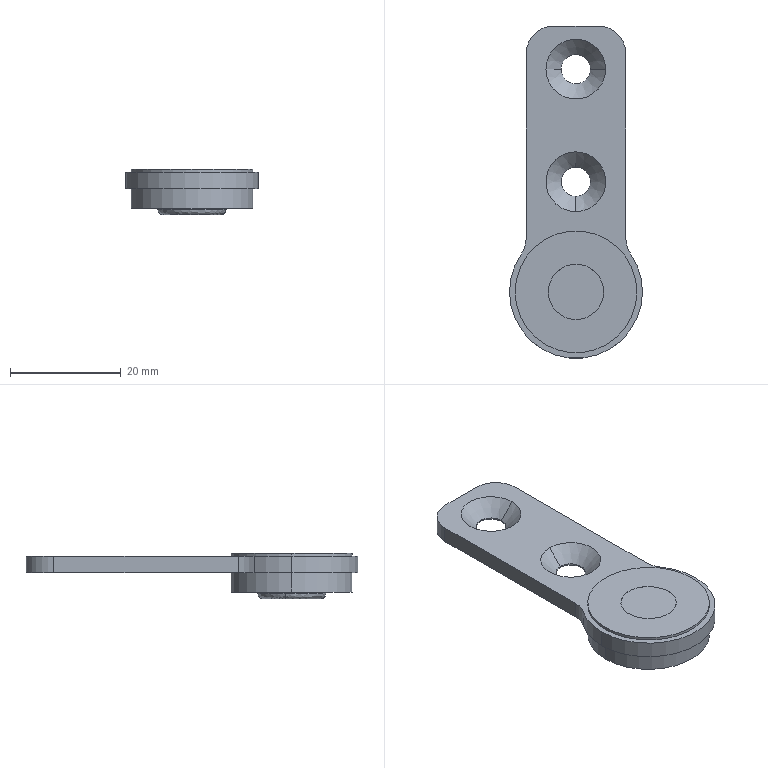Part | SolidWorks | features BaseBody 1 | 1 solid | 43 faces | box 24 x 60 x 8.2 mm | volume 4435 mm3 | cylinder 23 | plane 10 | cone 6 | spline 4 | commonest cylinder face diameters 10 x6 5.3 x4 22 x4 24 x3 7.6 x2 10.02 x2
STEP:
#1=CARTESIAN_POINT('',(-6.03,1.21,-3.8));
#2=VERTEX_POINT('',#1);
#3=CARTESIAN_POINT('',(-6.15,0.,-3.8));
#4=VERTEX_POINT('',#3);
#5=CARTESIAN_POINT('',(0.,0.,-3.8));
#6=DIRECTION('',(0.,0.,1.));
#7=DIRECTION('',(1.,0.,0.));
#8=AXIS2_PLACEMENT_3D('',#5,#6,#7);
#9=CIRCLE('',#8,6.15);
#10=EDGE_CURVE('',#2,#4,#9,.T.);
#11=ORIENTED_EDGE('',*,*,#10,.F.);
#12=CARTESIAN_POINT('',(-5.147,1.033,-4.7));
#13=VERTEX_POINT('',#12);
#14=CARTESIAN_POINT('',(-5.147,1.033,-3.8));
#15=DIRECTION('',(-0.1968,-0.9804,0.));
#16=DIRECTION('',(-0.9804,0.1968,0.));
#17=AXIS2_PLACEMENT_3D('',#14,#15,#16);
#18=CIRCLE('',#17,0.9);
#19=EDGE_CURVE('',#2,#13,#18,.T.);
#20=ORIENTED_EDGE('',*,*,#19,.T.);
#21=CARTESIAN_POINT('',(5.147,-1.033,-4.7));
#22=VERTEX_POINT('',#21);
#23=CARTESIAN_POINT('',(-5.147,1.033,-4.7));
#24=CARTESIAN_POINT('',(-7.214,-9.261,-4.7));
#25=CARTESIAN_POINT('',(3.081,-11.328,-4.7));
#26=CARTESIAN_POINT('',(5.147,-1.033,-4.7));
#27=(BOUNDED_CURVE()B_SPLINE_CURVE(3,(#23,#24,#25,#26),.UNSPECIFIED.,.F.,.F.)B_SPLINE_CURVE_WITH_KNOTS((4,4),(0.,1.),.UNSPECIFIED.)CURVE()GEOMETRIC_REPRESENTATION_ITEM()RATIONAL_B_SPLINE_CURVE((1.,0.3333,0.3333,1.))REPRESENTATION_ITEM(''));
#28=EDGE_CURVE('',#13,#22,#27,.T.);
#29=ORIENTED_EDGE('',*,*,#28,.T.);
#30=CARTESIAN_POINT('',(6.03,-1.21,-3.8));
#31=VERTEX_POINT('',#30);
#32=CARTESIAN_POINT('',(5.147,-1.033,-3.8));
#33=DIRECTION('',(0.1968,0.9804,0.));
#34=DIRECTION('',(0.9804,-0.1968,0.));
#35=AXIS2_PLACEMENT_3D('',#32,#33,#34);
#36=CIRCLE('',#35,0.9);
#37=EDGE_CURVE('',#31,#22,#36,.T.);
#38=ORIENTED_EDGE('',*,*,#37,.F.);
#39=CARTESIAN_POINT('',(0.,0.,-3.8));
#40=DIRECTION('',(0.,0.,1.));
#41=DIRECTION('',(1.,0.,0.));
#42=AXIS2_PLACEMENT_3D('',#39,#40,#41);
#43=CIRCLE('',#42,6.15);
#44=EDGE_CURVE('',#4,#31,#43,.T.);
#45=ORIENTED_EDGE('',*,*,#44,.F.);
#46=EDGE_LOOP('',(#11,#20,#29,#38,#45));
#47=FACE_OUTER_BOUND('',#46,.T.);
#48=CARTESIAN_POINT('',(-6.03,1.21,-3.8));
#49=CARTESIAN_POINT('',(-8.451,-10.849,-3.8));
#50=CARTESIAN_POINT('',(3.609,-13.27,-3.8));
#51=CARTESIAN_POINT('',(6.03,-1.21,-3.8));
#52=CARTESIAN_POINT('',(-6.03,1.21,-4.327));
#53=CARTESIAN_POINT('',(-8.451,-10.849,-4.327));
#54=CARTESIAN_POINT('',(3.609,-13.27,-4.327));
#55=CARTESIAN_POINT('',(6.03,-1.21,-4.327));
#56=CARTESIAN_POINT('',(-5.664,1.137,-4.7));
#57=CARTESIAN_POINT('',(-7.938,-10.191,-4.7));
#58=CARTESIAN_POINT('',(3.39,-12.465,-4.7));
#59=CARTESIAN_POINT('',(5.664,-1.137,-4.7));
#60=CARTESIAN_POINT('',(-5.147,1.033,-4.7));
#61=CARTESIAN_POINT('',(-7.214,-9.261,-4.7));
#62=CARTESIAN_POINT('',(3.081,-11.328,-4.7));
#63=CARTESIAN_POINT('',(5.147,-1.033,-4.7));
#64=(BOUNDED_SURFACE()B_SPLINE_SURFACE(3,3,((#48,#49,#50,#51),(#52,#53,#54,#55),(#56,#57,#58,#59),(#60,#61,#62,#63)),.UNSPECIFIED.,.F.,.F.,.F.)B_SPLINE_SURFACE_WITH_KNOTS((4,4),(4,4),(0.,1.),(0.,1.),.UNSPECIFIED.)GEOMETRIC_REPRESENTATION_ITEM()RATIONAL_B_SPLINE_SURFACE(((1.,0.3333,0.3333,1.),(0.8047,0.2682,0.2682,0.8047),(0.8047,0.2682,0.2682,0.8047),(1.,0.3333,0.3333,1.)))REPRESENTATION_ITEM('')SURFACE());
#65=ADVANCED_FACE('',(#47),#64,.T.);
#66=CARTESIAN_POINT('',(4.608,-0.925,-4.7));
#67=VERTEX_POINT('',#66);
#68=CARTESIAN_POINT('',(-4.608,0.925,-4.7));
#69=VERTEX_POINT('',#68);
#70=CARTESIAN_POINT('',(4.608,-0.925,-4.7));
#71=CARTESIAN_POINT('',(2.758,-10.141,-4.7));
#72=CARTESIAN_POINT('',(-6.458,-8.291,-4.7));
#73=CARTESIAN_POINT('',(-4.608,0.925,-4.7));
#74=(BOUNDED_CURVE()B_SPLINE_CURVE(3,(#70,#71,#72,#73),.UNSPECIFIED.,.F.,.F.)B_SPLINE_CURVE_WITH_KNOTS((4,4),(0.,1.),.UNSPECIFIED.)CURVE()GEOMETRIC_REPRESENTATION_ITEM()RATIONAL_B_SPLINE_CURVE((1.,0.3333,0.3333,1.))REPRESENTATION_ITEM(''));
#75=EDGE_CURVE('',#67,#69,#74,.T.);
#76=ORIENTED_EDGE('',*,*,#75,.T.);
#77=CARTESIAN_POINT('',(-3.726,0.7479,-3.8));
#78=VERTEX_POINT('',#77);
#79=CARTESIAN_POINT('',(-4.608,0.925,-3.8));
#80=DIRECTION('',(-0.1968,-0.9804,0.));
#81=DIRECTION('',(-0.9804,0.1968,0.));
#82=AXIS2_PLACEMENT_3D('',#79,#80,#81);
#83=CIRCLE('',#82,0.9);
#84=EDGE_CURVE('',#69,#78,#83,.T.);
#85=ORIENTED_EDGE('',*,*,#84,.T.);
#86=CARTESIAN_POINT('',(-3.8,0.,-3.8));
#87=VERTEX_POINT('',#86);
#88=CARTESIAN_POINT('',(0.,0.,-3.8));
#89=DIRECTION('',(0.,0.,1.));
#90=DIRECTION('',(0.9804,-0.1968,0.));
#91=AXIS2_PLACEMENT_3D('',#88,#89,#90);
#92=CIRCLE('',#91,3.8);
#93=EDGE_CURVE('',#78,#87,#92,.T.);
#94=ORIENTED_EDGE('',*,*,#93,.T.);
#95=CARTESIAN_POINT('',(3.726,-0.7479,-3.8));
#96=VERTEX_POINT('',#95);
#97=CARTESIAN_POINT('',(0.,0.,-3.8));
#98=DIRECTION('',(0.,0.,1.));
#99=DIRECTION('',(0.9804,-0.1968,0.));
#100=AXIS2_PLACEMENT_3D('',#97,#98,#99);
#101=CIRCLE('',#100,3.8);
#102=EDGE_CURVE('',#87,#96,#101,.T.);
#103=ORIENTED_EDGE('',*,*,#102,.T.);
#104=CARTESIAN_POINT('',(4.608,-0.925,-3.8));
#105=DIRECTION('',(0.1968,0.9804,0.));
#106=DIRECTION('',(0.9804,-0.1968,0.));
#107=AXIS2_PLACEMENT_3D('',#104,#105,#106);
#108=CIRCLE('',#107,0.9);
#109=EDGE_CURVE('',#67,#96,#108,.T.);
#110=ORIENTED_EDGE('',*,*,#109,.F.);
#111=EDGE_LOOP('',(#76,#85,#94,#103,#110));
#112=FACE_OUTER_BOUND('',#111,.T.);
#113=CARTESIAN_POINT('',(-4.608,0.925,-4.7));
#114=CARTESIAN_POINT('',(-6.458,-8.291,-4.7));
#115=CARTESIAN_POINT('',(2.758,-10.141,-4.7));
#116=CARTESIAN_POINT('',(4.608,-0.925,-4.7));
#117=CARTESIAN_POINT('',(-4.091,0.8213,-4.7));
#118=CARTESIAN_POINT('',(-5.734,-7.361,-4.7));
#119=CARTESIAN_POINT('',(2.449,-9.004,-4.7));
#120=CARTESIAN_POINT('',(4.091,-0.8213,-4.7));
#121=CARTESIAN_POINT('',(-3.726,0.7479,-4.327));
#122=CARTESIAN_POINT('',(-5.221,-6.703,-4.327));
#123=CARTESIAN_POINT('',(2.23,-8.199,-4.327));
#124=CARTESIAN_POINT('',(3.726,-0.7479,-4.327));
#125=CARTESIAN_POINT('',(-3.726,0.7479,-3.8));
#126=CARTESIAN_POINT('',(-5.221,-6.703,-3.8));
#127=CARTESIAN_POINT('',(2.23,-8.199,-3.8));
#128=CARTESIAN_POINT('',(3.726,-0.7479,-3.8));
#129=(BOUNDED_SURFACE()B_SPLINE_SURFACE(3,3,((#113,#114,#115,#116),(#117,#118,#119,#120),(#121,#122,#123,#124),(#125,#126,#127,#128)),.UNSPECIFIED.,.F.,.F.,.T.)B_SPLINE_SURFACE_WITH_KNOTS((4,4),(4,4),(0.,1.),(0.,1.),.UNSPECIFIED.)GEOMETRIC_REPRESENTATION_ITEM()RATIONAL_B_SPLINE_SURFACE(((1.,0.3333,0.3333,1.),(0.8047,0.2682,0.2682,0.8047),(0.8047,0.2682,0.2682,0.8047),(1.,0.3333,0.3333,1.)))REPRESENTATION_ITEM('')SURFACE());
#130=ADVANCED_FACE('',(#112),#129,.T.);
#131=CARTESIAN_POINT('',(2.612,40.201,0.));
#132=VERTEX_POINT('',#131);
#133=CARTESIAN_POINT('',(-2.688,40.201,0.));
#134=VERTEX_POINT('',#133);
#135=CARTESIAN_POINT('',(-0.03816,40.201,0.));
#136=DIRECTION('',(0.,0.,-1.));
#137=DIRECTION('',(1.,0.,0.));
#138=AXIS2_PLACEMENT_3D('',#135,#136,#137);
#139=CIRCLE('',#138,2.65);
#140=EDGE_CURVE('',#132,#134,#139,.T.);
#141=ORIENTED_EDGE('',*,*,#140,.T.);
#142=CARTESIAN_POINT('',(-2.688,40.201,0.25));
#143=VERTEX_POINT('',#142);
#144=CARTESIAN_POINT('',(-2.688,40.201,3.));
#145=DIRECTION('',(0.,0.,1.));
#146=VECTOR('',#145,1000.);
#147=LINE('',#144,#146);
#148=EDGE_CURVE('',#134,#143,#147,.T.);
#149=ORIENTED_EDGE('',*,*,#148,.T.);
#150=CARTESIAN_POINT('',(2.612,40.201,0.25));
#151=VERTEX_POINT('',#150);
#152=CARTESIAN_POINT('',(-0.03816,40.201,0.25));
#153=DIRECTION('',(0.,0.,-1.));
#154=DIRECTION('',(1.,0.,0.));
#155=AXIS2_PLACEMENT_3D('',#152,#153,#154);
#156=CIRCLE('',#155,2.65);
#157=EDGE_CURVE('',#151,#143,#156,.T.);
#158=ORIENTED_EDGE('',*,*,#157,.F.);
#159=CARTESIAN_POINT('',(2.612,40.201,3.));
#160=DIRECTION('',(0.,0.,1.));
#161=VECTOR('',#160,1000.);
#162=LINE('',#159,#161);
#163=EDGE_CURVE('',#132,#151,#162,.T.);
#164=ORIENTED_EDGE('',*,*,#163,.F.);
#165=EDGE_LOOP('',(#141,#149,#158,#164));
#166=FACE_OUTER_BOUND('',#165,.T.);
#167=CARTESIAN_POINT('',(-0.03816,40.201,3.));
#168=DIRECTION('',(0.,0.,1.));
#169=DIRECTION('',(1.,0.,0.));
#170=AXIS2_PLACEMENT_3D('',#167,#168,#169);
#171=CYLINDRICAL_SURFACE('',#170,2.65);
#172=ADVANCED_FACE('',(#166),#171,.F.);
#173=CARTESIAN_POINT('',(2.619,19.883,0.));
#174=VERTEX_POINT('',#173);
#175=CARTESIAN_POINT('',(-2.681,19.883,0.));
#176=VERTEX_POINT('',#175);
#177=CARTESIAN_POINT('',(-0.03149,19.883,0.));
#178=DIRECTION('',(0.,0.,-1.));
#179=DIRECTION('',(1.,0.,0.));
#180=AXIS2_PLACEMENT_3D('',#177,#178,#179);
#181=CIRCLE('',#180,2.65);
#182=EDGE_CURVE('',#174,#176,#181,.T.);
#183=ORIENTED_EDGE('',*,*,#182,.T.);
#184=CARTESIAN_POINT('',(-2.681,19.883,0.25));
#185=VERTEX_POINT('',#184);
#186=CARTESIAN_POINT('',(-2.681,19.883,3.));
#187=DIRECTION('',(0.,0.,1.));
#188=VECTOR('',#187,1000.);
#189=LINE('',#186,#188);
#190=EDGE_CURVE('',#176,#185,#189,.T.);
#191=ORIENTED_EDGE('',*,*,#190,.T.);
#192=CARTESIAN_POINT('',(-0.03149,17.233,0.25));
#193=VERTEX_POINT('',#192);
#194=CARTESIAN_POINT('',(-0.03149,19.883,0.25));
#195=DIRECTION('',(0.,0.,-1.));
#196=DIRECTION('',(1.,0.,0.));
#197=AXIS2_PLACEMENT_3D('',#194,#195,#196);
#198=CIRCLE('',#197,2.65);
#199=EDGE_CURVE('',#193,#185,#198,.T.);
#200=ORIENTED_EDGE('',*,*,#199,.F.);
#201=CARTESIAN_POINT('',(2.619,19.883,0.25));
#202=VERTEX_POINT('',#201);
#203=CARTESIAN_POINT('',(-0.03149,19.883,0.25));
#204=DIRECTION('',(0.,0.,-1.));
#205=DIRECTION('',(1.,0.,0.));
#206=AXIS2_PLACEMENT_3D('',#203,#204,#205);
#207=CIRCLE('',#206,2.65);
#208=EDGE_CURVE('',#202,#193,#207,.T.);
#209=ORIENTED_EDGE('',*,*,#208,.F.);
#210=CARTESIAN_POINT('',(2.619,19.883,3.));
#211=DIRECTION('',(0.,0.,1.));
#212=VECTOR('',#211,1000.);
#213=LINE('',#210,#212);
#214=EDGE_CURVE('',#174,#202,#213,.T.);
#215=ORIENTED_EDGE('',*,*,#214,.F.);
#216=EDGE_LOOP('',(#183,#191,#200,#209,#215));
#217=FACE_OUTER_BOUND('',#216,.T.);
#218=CARTESIAN_POINT('',(-0.03149,19.883,3.));
#219=DIRECTION('',(0.,0.,1.));
#220=DIRECTION('',(1.,0.,0.));
#221=AXIS2_PLACEMENT_3D('',#218,#219,#220);
#222=CYLINDRICAL_SURFACE('',#221,2.65);
#223=ADVANCED_FACE('',(#217),#222,.F.);
#224=CARTESIAN_POINT('',(9.882,6.807,3.));
#225=VERTEX_POINT('',#224);
#226=CARTESIAN_POINT('',(12.,0.,3.));
#227=VERTEX_POINT('',#226);
#228=CARTESIAN_POINT('',(0.,0.,3.));
#229=DIRECTION('',(0.,0.,-1.));
#230=DIRECTION('',(-1.,0.,0.));
#231=AXIS2_PLACEMENT_3D('',#228,#229,#230);
#232=CIRCLE('',#231,12.);
#233=EDGE_CURVE('',#225,#227,#232,.T.);
#234=ORIENTED_EDGE('',*,*,#233,.T.);
#235=CARTESIAN_POINT('',(12.,0.,0.));
#236=VERTEX_POINT('',#235);
#237=CARTESIAN_POINT('',(12.,0.,3.));
#238=DIRECTION('',(0.,0.,-1.));
#239=VECTOR('',#238,1000.);
#240=LINE('',#237,#239);
#241=EDGE_CURVE('',#227,#236,#240,.T.);
#242=ORIENTED_EDGE('',*,*,#241,.T.);
#243=CARTESIAN_POINT('',(9.882,6.807,0.));
#244=VERTEX_POINT('',#243);
#245=CARTESIAN_POINT('',(0.,0.,0.));
#246=DIRECTION('',(0.,0.,1.));
#247=DIRECTION('',(-1.,0.,0.));
#248=AXIS2_PLACEMENT_3D('',#245,#246,#247);
#249=CIRCLE('',#248,12.);
#250=EDGE_CURVE('',#236,#244,#249,.T.);
#251=ORIENTED_EDGE('',*,*,#250,.T.);
#252=CARTESIAN_POINT('',(9.882,6.807,3.));
#253=DIRECTION('',(0.,0.,1.));
#254=VECTOR('',#253,1000.);
#255=LINE('',#252,#254);
#256=EDGE_CURVE('',#244,#225,#255,.T.);
#257=ORIENTED_EDGE('',*,*,#256,.T.);
#258=EDGE_LOOP('',(#234,#242,#251,#257));
#259=FACE_OUTER_BOUND('',#258,.T.);
#260=CARTESIAN_POINT('',(0.,0.,3.));
#261=DIRECTION('',(0.,0.,-1.));
#262=DIRECTION('',(-1.,0.,0.));
#263=AXIS2_PLACEMENT_3D('',#260,#261,#262);
#264=CYLINDRICAL_SURFACE('',#263,12.);
#265=ADVANCED_FACE('',(#259),#264,.T.);
#266=ORIENTED_EDGE('',*,*,#241,.F.);
#267=CARTESIAN_POINT('',(-12.,0.,3.));
#268=VERTEX_POINT('',#267);
#269=CARTESIAN_POINT('',(0.,0.,3.));
#270=DIRECTION('',(0.,0.,-1.));
#271=DIRECTION('',(-1.,0.,0.));
#272=AXIS2_PLACEMENT_3D('',#269,#270,#271);
#273=CIRCLE('',#272,12.);
#274=EDGE_CURVE('',#227,#268,#273,.T.);
#275=ORIENTED_EDGE('',*,*,#274,.T.);
#276=CARTESIAN_POINT('',(-12.,0.,0.));
#277=VERTEX_POINT('',#276);
#278=CARTESIAN_POINT('',(-12.,0.,3.));
#279=DIRECTION('',(0.,0.,-1.));
#280=VECTOR('',#279,1000.);
#281=LINE('',#278,#280);
#282=EDGE_CURVE('',#268,#277,#281,.T.);
#283=ORIENTED_EDGE('',*,*,#282,.T.);
#284=CARTESIAN_POINT('',(0.,0.,0.));
#285=DIRECTION('',(0.,0.,1.));
#286=DIRECTION('',(-1.,0.,0.));
#287=AXIS2_PLACEMENT_3D('',#284,#285,#286);
#288=CIRCLE('',#287,12.);
#289=EDGE_CURVE('',#277,#236,#288,.T.);
#290=ORIENTED_EDGE('',*,*,#289,.T.);
#291=EDGE_LOOP('',(#266,#275,#283,#290));
#292=FACE_OUTER_BOUND('',#291,.T.);
#293=CARTESIAN_POINT('',(0.,0.,3.));
#294=DIRECTION('',(0.,0.,-1.));
#295=DIRECTION('',(-1.,0.,0.));
#296=AXIS2_PLACEMENT_3D('',#293,#294,#295);
#297=CYLINDRICAL_SURFACE('',#296,12.);
#298=ADVANCED_FACE('',(#292),#297,.T.);
#299=CARTESIAN_POINT('',(-11.,0.,0.));
#300=VERTEX_POINT('',#299);
#301=CARTESIAN_POINT('',(11.,0.,0.));
#302=VERTEX_POINT('',#301);
#303=CARTESIAN_POINT('',(0.,0.,0.));
#304=DIRECTION('',(0.,0.,-1.));
#305=DIRECTION('',(-1.,0.,0.));
#306=AXIS2_PLACEMENT_3D('',#303,#304,#305);
#307=CIRCLE('',#306,11.);
#308=EDGE_CURVE('',#300,#302,#307,.T.);
#309=ORIENTED_EDGE('',*,*,#308,.T.);
#310=CARTESIAN_POINT('',(11.,0.,-3.5));
#311=VERTEX_POINT('',#310);
#312=CARTESIAN_POINT('',(11.,0.,0.));
#313=DIRECTION('',(0.,0.,-1.));
#314=VECTOR('',#313,1000.);
#315=LINE('',#312,#314);
#316=EDGE_CURVE('',#302,#311,#315,.T.);
#317=ORIENTED_EDGE('',*,*,#316,.T.);
#318=CARTESIAN_POINT('',(-11.,0.,-3.5));
#319=VERTEX_POINT('',#318);
#320=CARTESIAN_POINT('',(0.,0.,-3.5));
#321=DIRECTION('',(0.,0.,1.));
#322=DIRECTION('',(-1.,0.,0.));
#323=AXIS2_PLACEMENT_3D('',#320,#321,#322);
#324=CIRCLE('',#323,11.);
#325=EDGE_CURVE('',#311,#319,#324,.T.);
#326=ORIENTED_EDGE('',*,*,#325,.T.);
#327=CARTESIAN_POINT('',(-11.,0.,0.));
#328=DIRECTION('',(0.,0.,-1.));
#329=VECTOR('',#328,1000.);
#330=LINE('',#327,#329);
#331=EDGE_CURVE('',#300,#319,#330,.T.);
#332=ORIENTED_EDGE('',*,*,#331,.F.);
#333=EDGE_LOOP('',(#309,#317,#326,#332));
#334=FACE_OUTER_BOUND('',#333,.T.);
#335=CARTESIAN_POINT('',(0.,0.,0.));
#336=DIRECTION('',(0.,0.,-1.));
#337=DIRECTION('',(-1.,0.,0.));
#338=AXIS2_PLACEMENT_3D('',#335,#336,#337);
#339=CYLINDRICAL_SURFACE('',#338,11.);
#340=ADVANCED_FACE('',(#334),#339,.T.);
#341=ORIENTED_EDGE('',*,*,#157,.T.);
#342=CARTESIAN_POINT('',(-5.438,40.201,3.));
#343=VERTEX_POINT('',#342);
#344=CARTESIAN_POINT('',(-5.438,40.201,3.));
#345=DIRECTION('',(-0.7071,0.,0.7071));
#346=VECTOR('',#345,1000.);
#347=LINE('',#344,#346);
#348=EDGE_CURVE('',#143,#343,#347,.T.);
#349=ORIENTED_EDGE('',*,*,#348,.T.);
#350=CARTESIAN_POINT('',(5.362,40.201,3.));
#351=VERTEX_POINT('',#350);
#352=CARTESIAN_POINT('',(-0.03816,40.201,3.));
#353=DIRECTION('',(0.,0.,-1.));
#354=DIRECTION('',(1.,0.,0.));
#355=AXIS2_PLACEMENT_3D('',#352,#353,#354);
#356=CIRCLE('',#355,5.4);
#357=EDGE_CURVE('',#351,#343,#356,.T.);
#358=ORIENTED_EDGE('',*,*,#357,.F.);
#359=CARTESIAN_POINT('',(5.362,40.201,3.));
#360=DIRECTION('',(0.7071,0.,0.7071));
#361=VECTOR('',#360,1000.);
#362=LINE('',#359,#361);
#363=EDGE_CURVE('',#151,#351,#362,.T.);
#364=ORIENTED_EDGE('',*,*,#363,.F.);
#365=EDGE_LOOP('',(#341,#349,#358,#364));
#366=FACE_OUTER_BOUND('',#365,.T.);
#367=CARTESIAN_POINT('',(-0.03816,40.201,3.));
#368=DIRECTION('',(0.,0.,1.));
#369=DIRECTION('',(1.,0.,0.));
#370=AXIS2_PLACEMENT_3D('',#367,#368,#369);
#371=CONICAL_SURFACE('',#370,5.4,0.7854);
#372=ADVANCED_FACE('',(#366),#371,.F.);
#373=ORIENTED_EDGE('',*,*,#199,.T.);
#374=CARTESIAN_POINT('',(-0.03149,22.533,0.25));
#375=VERTEX_POINT('',#374);
#376=CARTESIAN_POINT('',(-0.03149,19.883,0.25));
#377=DIRECTION('',(0.,0.,-1.));
#378=DIRECTION('',(1.,0.,0.));
#379=AXIS2_PLACEMENT_3D('',#376,#377,#378);
#380=CIRCLE('',#379,2.65);
#381=EDGE_CURVE('',#185,#375,#380,.T.);
#382=ORIENTED_EDGE('',*,*,#381,.T.);
#383=CARTESIAN_POINT('',(-0.03149,25.283,3.));
#384=VERTEX_POINT('',#383);
#385=CARTESIAN_POINT('',(-0.03149,25.283,3.));
#386=DIRECTION('',(0.,0.7071,0.7071));
#387=VECTOR('',#386,1000.);
#388=LINE('',#385,#387);
#389=EDGE_CURVE('',#375,#384,#388,.T.);
#390=ORIENTED_EDGE('',*,*,#389,.T.);
#391=CARTESIAN_POINT('',(-0.03149,14.483,3.));
#392=VERTEX_POINT('',#391);
#393=CARTESIAN_POINT('',(-0.03149,19.883,3.));
#394=DIRECTION('',(0.,0.,-1.));
#395=DIRECTION('',(0.,-1.,0.));
#396=AXIS2_PLACEMENT_3D('',#393,#394,#395);
#397=CIRCLE('',#396,5.4);
#398=EDGE_CURVE('',#392,#384,#397,.T.);
#399=ORIENTED_EDGE('',*,*,#398,.F.);
#400=CARTESIAN_POINT('',(-0.03149,14.483,3.));
#401=DIRECTION('',(0.,-0.7071,0.7071));
#402=VECTOR('',#401,1000.);
#403=LINE('',#400,#402);
#404=EDGE_CURVE('',#193,#392,#403,.T.);
#405=ORIENTED_EDGE('',*,*,#404,.F.);
#406=EDGE_LOOP('',(#373,#382,#390,#399,#405));
#407=FACE_OUTER_BOUND('',#406,.T.);
#408=CARTESIAN_POINT('',(-0.03149,19.883,3.));
#409=DIRECTION('',(0.,0.,1.));
#410=DIRECTION('',(0.,-1.,0.));
#411=AXIS2_PLACEMENT_3D('',#408,#409,#410);
#412=CONICAL_SURFACE('',#411,5.4,0.7854);
#413=ADVANCED_FACE('',(#407),#412,.F.);
#414=CARTESIAN_POINT('',(-11.,0.,3.5));
#415=VERTEX_POINT('',#414);
#416=CARTESIAN_POINT('',(11.,0.,3.5));
#417=VERTEX_POINT('',#416);
#418=CARTESIAN_POINT('',(0.,0.,3.5));
#419=DIRECTION('',(0.,0.,-1.));
#420=DIRECTION('',(-1.,0.,0.));
#421=AXIS2_PLACEMENT_3D('',#418,#419,#420);
#422=CIRCLE('',#421,11.);
#423=EDGE_CURVE('',#415,#417,#422,.T.);
#424=ORIENTED_EDGE('',*,*,#423,.T.);
#425=CARTESIAN_POINT('',(11.,0.,3.));
#426=VERTEX_POINT('',#425);
#427=CARTESIAN_POINT('',(11.,0.,3.5));
#428=DIRECTION('',(0.,0.,-1.));
#429=VECTOR('',#428,1000.);
#430=LINE('',#427,#429);
#431=EDGE_CURVE('',#417,#426,#430,.T.);
#432=ORIENTED_EDGE('',*,*,#431,.T.);
#433=CARTESIAN_POINT('',(-11.,0.,3.));
#434=VERTEX_POINT('',#433);
#435=CARTESIAN_POINT('',(0.,0.,3.));
#436=DIRECTION('',(0.,0.,-1.));
#437=DIRECTION('',(-1.,0.,0.));
#438=AXIS2_PLACEMENT_3D('',#435,#436,#437);
#439=CIRCLE('',#438,11.);
#440=EDGE_CURVE('',#434,#426,#439,.T.);
#441=ORIENTED_EDGE('',*,*,#440,.F.);
#442=CARTESIAN_POINT('',(-11.,0.,3.5));
#443=DIRECTION('',(0.,0.,-1.));
#444=VECTOR('',#443,1000.);
#445=LINE('',#442,#444);
#446=EDGE_CURVE('',#415,#434,#445,.T.);
#447=ORIENTED_EDGE('',*,*,#446,.F.);
#448=EDGE_LOOP('',(#424,#432,#441,#447));
#449=FACE_OUTER_BOUND('',#448,.T.);
#450=CARTESIAN_POINT('',(0.,0.,3.5));
#451=DIRECTION('',(0.,0.,-1.));
#452=DIRECTION('',(-1.,0.,0.));
#453=AXIS2_PLACEMENT_3D('',#450,#451,#452);
#454=CYLINDRICAL_SURFACE('',#453,11.);
#455=ADVANCED_FACE('',(#449),#454,.T.);
#456=CARTESIAN_POINT('',(6.15,0.,-3.8));
#457=VERTEX_POINT('',#456);
#458=CARTESIAN_POINT('',(0.,0.,-3.8));
#459=DIRECTION('',(0.,0.,1.));
#460=DIRECTION('',(1.,0.,0.));
#461=AXIS2_PLACEMENT_3D('',#458,#459,#460);
#462=CIRCLE('',#461,6.15);
#463=EDGE_CURVE('',#457,#2,#462,.T.);
#464=ORIENTED_EDGE('',*,*,#463,.T.);
#465=ORIENTED_EDGE('',*,*,#10,.T.);
#466=CARTESIAN_POINT('',(-6.15,0.,-3.5));
#467=VERTEX_POINT('',#466);
#468=CARTESIAN_POINT('',(-6.15,0.,60.062));
#469=DIRECTION('',(0.,0.,1.));
#470=VECTOR('',#469,1000.);
#471=LINE('',#468,#470);
#472=EDGE_CURVE('',#4,#467,#471,.T.);
#473=ORIENTED_EDGE('',*,*,#472,.T.);
#474=CARTESIAN_POINT('',(6.15,0.,-3.5));
#475=VERTEX_POINT('',#474);
#476=CARTESIAN_POINT('',(0.,0.,-3.5));
#477=DIRECTION('',(0.,0.,-1.));
#478=DIRECTION('',(1.,0.,0.));
#479=AXIS2_PLACEMENT_3D('',#476,#477,#478);
#480=CIRCLE('',#479,6.15);
#481=EDGE_CURVE('',#467,#475,#480,.T.);
#482=ORIENTED_EDGE('',*,*,#481,.T.);
#483=CARTESIAN_POINT('',(6.15,0.,60.062));
#484=DIRECTION('',(0.,0.,1.));
#485=VECTOR('',#484,1000.);
#486=LINE('',#483,#485);
#487=EDGE_CURVE('',#457,#475,#486,.T.);
#488=ORIENTED_EDGE('',*,*,#487,.F.);
#489=EDGE_LOOP('',(#464,#465,#473,#482,#488));
#490=FACE_OUTER_BOUND('',#489,.T.);
#491=CARTESIAN_POINT('',(0.,0.,60.062));
#492=DIRECTION('',(0.,0.,1.));
#493=DIRECTION('',(1.,0.,0.));
#494=AXIS2_PLACEMENT_3D('',#491,#492,#493);
#495=CYLINDRICAL_SURFACE('',#494,6.15);
#496=ADVANCED_FACE('',(#490),#495,.T.);
#497=CARTESIAN_POINT('',(-5.01,0.,-3.5));
#498=VERTEX_POINT('',#497);
#499=CARTESIAN_POINT('',(5.01,0.,-3.5));
#500=VERTEX_POINT('',#499);
#501=CARTESIAN_POINT('',(0.,0.,-3.5));
#502=DIRECTION('',(0.,0.,1.));
#503=DIRECTION('',(1.,0.,0.));
#504=AXIS2_PLACEMENT_3D('',#501,#502,#503);
#505=CIRCLE('',#504,5.01);
#506=EDGE_CURVE('',#498,#500,#505,.T.);
#507=ORIENTED_EDGE('',*,*,#506,.F.);
#508=CARTESIAN_POINT('',(-5.01,0.,3.5));
#509=VERTEX_POINT('',#508);
#510=CARTESIAN_POINT('',(-5.01,0.,3.));
#511=DIRECTION('',(0.,0.,1.));
#512=VECTOR('',#511,1000.);
#513=LINE('',#510,#512);
#514=EDGE_CURVE('',#498,#509,#513,.T.);
#515=ORIENTED_EDGE('',*,*,#514,.T.);
#516=CARTESIAN_POINT('',(5.01,0.,3.5));
#517=VERTEX_POINT('',#516);
#518=CARTESIAN_POINT('',(0.,0.,3.5));
#519=DIRECTION('',(0.,0.,-1.));
#520=DIRECTION('',(1.,0.,0.));
#521=AXIS2_PLACEMENT_3D('',#518,#519,#520);
#522=CIRCLE('',#521,5.01);
#523=EDGE_CURVE('',#517,#509,#522,.T.);
#524=ORIENTED_EDGE('',*,*,#523,.F.);
#525=CARTESIAN_POINT('',(5.01,0.,3.));
#526=DIRECTION('',(0.,0.,1.));
#527=VECTOR('',#526,1000.);
#528=LINE('',#525,#527);
#529=EDGE_CURVE('',#500,#517,#528,.T.);
#530=ORIENTED_EDGE('',*,*,#529,.F.);
#531=EDGE_LOOP('',(#507,#515,#524,#530));
#532=FACE_OUTER_BOUND('',#531,.T.);
#533=CARTESIAN_POINT('',(0.,0.,3.));
#534=DIRECTION('',(0.,0.,1.));
#535=DIRECTION('',(1.,0.,0.));
#536=AXIS2_PLACEMENT_3D('',#533,#534,#535);
#537=CYLINDRICAL_SURFACE('',#536,5.01);
#538=ADVANCED_FACE('',(#532),#537,.F.);
#539=CARTESIAN_POINT('',(5.,0.,-3.5));
#540=VERTEX_POINT('',#539);
#541=CARTESIAN_POINT('',(-5.,0.,-3.5));
#542=VERTEX_POINT('',#541);
#543=CARTESIAN_POINT('',(0.,0.,-3.5));
#544=DIRECTION('',(0.,0.,1.));
#545=DIRECTION('',(1.,0.,0.));
#546=AXIS2_PLACEMENT_3D('',#543,#544,#545);
#547=CIRCLE('',#546,5.);
#548=EDGE_CURVE('',#540,#542,#547,.T.);
#549=ORIENTED_EDGE('',*,*,#548,.T.);
#550=CARTESIAN_POINT('',(-5.,0.,3.5));
#551=VERTEX_POINT('',#550);
#552=CARTESIAN_POINT('',(-5.,0.,60.062));
#553=DIRECTION('',(0.,0.,1.));
#554=VECTOR('',#553,1000.);
#555=LINE('',#552,#554);
#556=EDGE_CURVE('',#542,#551,#555,.T.);
#557=ORIENTED_EDGE('',*,*,#556,.T.);
#558=CARTESIAN_POINT('',(5.,0.,3.5));
#559=VERTEX_POINT('',#558);
#560=CARTESIAN_POINT('',(0.,0.,3.5));
#561=DIRECTION('',(0.,0.,-1.));
#562=DIRECTION('',(1.,0.,0.));
#563=AXIS2_PLACEMENT_3D('',#560,#561,#562);
#564=CIRCLE('',#563,5.);
#565=EDGE_CURVE('',#551,#559,#564,.T.);
#566=ORIENTED_EDGE('',*,*,#565,.T.);
#567=CARTESIAN_POINT('',(5.,0.,60.062));
#568=DIRECTION('',(0.,0.,1.));
#569=VECTOR('',#568,1000.);
#570=LINE('',#567,#569);
#571=EDGE_CURVE('',#540,#559,#570,.T.);
#572=ORIENTED_EDGE('',*,*,#571,.F.);
#573=EDGE_LOOP('',(#549,#557,#566,#572));
#574=FACE_OUTER_BOUND('',#573,.T.);
#575=CARTESIAN_POINT('',(0.,0.,60.062));
#576=DIRECTION('',(0.,0.,1.));
#577=DIRECTION('',(1.,0.,0.));
#578=AXIS2_PLACEMENT_3D('',#575,#576,#577);
#579=CYLINDRICAL_SURFACE('',#578,5.);
#580=ADVANCED_FACE('',(#574),#579,.T.);
#581=ORIENTED_EDGE('',*,*,#102,.F.);
#582=CARTESIAN_POINT('',(-3.8,0.,0.1));
#583=VERTEX_POINT('',#582);
#584=CARTESIAN_POINT('',(-3.8,0.,60.062));
#585=DIRECTION('',(0.,0.,1.));
#586=VECTOR('',#585,1000.);
#587=LINE('',#584,#586);
#588=EDGE_CURVE('',#87,#583,#587,.T.);
#589=ORIENTED_EDGE('',*,*,#588,.T.);
#590=CARTESIAN_POINT('',(3.8,0.,0.1));
#591=VERTEX_POINT('',#590);
#592=CARTESIAN_POINT('',(0.,0.,0.1));
#593=DIRECTION('',(0.,0.,-1.));
#594=DIRECTION('',(1.,0.,0.));
#595=AXIS2_PLACEMENT_3D('',#592,#593,#594);
#596=CIRCLE('',#595,3.8);
#597=EDGE_CURVE('',#591,#583,#596,.T.);
#598=ORIENTED_EDGE('',*,*,#597,.F.);
#599=CARTESIAN_POINT('',(3.8,0.,-3.8));
#600=VERTEX_POINT('',#599);
#601=CARTESIAN_POINT('',(3.8,0.,60.062));
#602=DIRECTION('',(0.,0.,1.));
#603=VECTOR('',#602,1000.);
#604=LINE('',#601,#603);
#605=EDGE_CURVE('',#600,#591,#604,.T.);
#606=ORIENTED_EDGE('',*,*,#605,.F.);
#607=CARTESIAN_POINT('',(0.,0.,-3.8));
#608=DIRECTION('',(0.,0.,1.));
#609=DIRECTION('',(0.9804,-0.1968,0.));
#610=AXIS2_PLACEMENT_3D('',#607,#608,#609);
#611=CIRCLE('',#610,3.8);
#612=EDGE_CURVE('',#96,#600,#611,.T.);
#613=ORIENTED_EDGE('',*,*,#612,.F.);
#614=EDGE_LOOP('',(#581,#589,#598,#606,#613));
#615=FACE_OUTER_BOUND('',#614,.T.);
#616=CARTESIAN_POINT('',(0.,0.,60.062));
#617=DIRECTION('',(0.,0.,1.));
#618=DIRECTION('',(1.,0.,0.));
#619=AXIS2_PLACEMENT_3D('',#616,#617,#618);
#620=CYLINDRICAL_SURFACE('',#619,3.8);
#621=ADVANCED_FACE('',(#615),#620,.F.);
#622=CARTESIAN_POINT('',(0.,0.,2.294));
#623=VERTEX_POINT('',#622);
#624=CARTESIAN_POINT('',(-3.8,0.,0.1));
#625=DIRECTION('',(-0.866,0.,-0.5));
#626=VECTOR('',#625,1000.);
#627=LINE('',#624,#626);
#628=EDGE_CURVE('',#623,#583,#627,.T.);
#629=ORIENTED_EDGE('',*,*,#628,.F.);
#630=CARTESIAN_POINT('',(3.8,0.,0.1));
#631=DIRECTION('',(0.866,0.,-0.5));
#632=VECTOR('',#631,1000.);
#633=LINE('',#630,#632);
#634=EDGE_CURVE('',#623,#591,#633,.T.);
#635=ORIENTED_EDGE('',*,*,#634,.T.);
#636=ORIENTED_EDGE('',*,*,#597,.T.);
#637=EDGE_LOOP('',(#629,#635,#636));
#638=FACE_OUTER_BOUND('',#637,.T.);
#639=CARTESIAN_POINT('',(0.,0.,0.1));
#640=DIRECTION('',(0.,0.,-1.));
#641=DIRECTION('',(-1.,0.,0.));
#642=AXIS2_PLACEMENT_3D('',#639,#640,#641);
#643=CONICAL_SURFACE('',#642,3.8,1.047);
#644=ADVANCED_FACE('',(#638),#643,.F.);
#645=ORIENTED_EDGE('',*,*,#140,.F.);
#646=CARTESIAN_POINT('',(-0.03816,40.201,0.));
#647=DIRECTION('',(0.,0.,-1.));
#648=DIRECTION('',(1.,0.,0.));
#649=AXIS2_PLACEMENT_3D('',#646,#647,#648);
#650=CIRCLE('',#649,2.65);
#651=EDGE_CURVE('',#134,#132,#650,.T.);
#652=ORIENTED_EDGE('',*,*,#651,.F.);
#653=EDGE_LOOP('',(#645,#652));
#654=FACE_BOUND('',#653,.T.);
#655=ORIENTED_EDGE('',*,*,#182,.F.);
#656=CARTESIAN_POINT('',(-0.03149,19.883,0.));
#657=DIRECTION('',(0.,0.,-1.));
#658=DIRECTION('',(1.,0.,0.));
#659=AXIS2_PLACEMENT_3D('',#656,#657,#658);
#660=CIRCLE('',#659,2.65);
#661=EDGE_CURVE('',#176,#174,#660,.T.);
#662=ORIENTED_EDGE('',*,*,#661,.F.);
#663=EDGE_LOOP('',(#655,#662));
#664=FACE_BOUND('',#663,.T.);
#665=CARTESIAN_POINT('',(-9.,9.644,0.));
#666=VERTEX_POINT('',#665);
#667=CARTESIAN_POINT('',(-9.882,6.807,0.));
#668=VERTEX_POINT('',#667);
#669=CARTESIAN_POINT('',(-14.,9.644,0.));
#670=DIRECTION('',(0.,0.,-1.));
#671=DIRECTION('',(-1.,0.,0.));
#672=AXIS2_PLACEMENT_3D('',#669,#670,#671);
#673=CIRCLE('',#672,5.);
#674=EDGE_CURVE('',#666,#668,#673,.T.);
#675=ORIENTED_EDGE('',*,*,#674,.F.);
#676=CARTESIAN_POINT('',(-9.,43.,0.));
#677=VERTEX_POINT('',#676);
#678=CARTESIAN_POINT('',(-9.,0.,0.));
#679=DIRECTION('',(0.,-1.,0.));
#680=VECTOR('',#679,1000.);
#681=LINE('',#678,#680);
#682=EDGE_CURVE('',#677,#666,#681,.T.);
#683=ORIENTED_EDGE('',*,*,#682,.F.);
#684=CARTESIAN_POINT('',(-4.,48.,0.));
#685=VERTEX_POINT('',#684);
#686=CARTESIAN_POINT('',(-4.,43.,0.));
#687=DIRECTION('',(0.,0.,1.));
#688=DIRECTION('',(-1.,0.,0.));
#689=AXIS2_PLACEMENT_3D('',#686,#687,#688);
#690=CIRCLE('',#689,5.);
#691=EDGE_CURVE('',#685,#677,#690,.T.);
#692=ORIENTED_EDGE('',*,*,#691,.F.);
#693=CARTESIAN_POINT('',(4.,48.,0.));
#694=VERTEX_POINT('',#693);
#695=CARTESIAN_POINT('',(0.,48.,0.));
#696=DIRECTION('',(-1.,0.,0.));
#697=VECTOR('',#696,1000.);
#698=LINE('',#695,#697);
#699=EDGE_CURVE('',#694,#685,#698,.T.);
#700=ORIENTED_EDGE('',*,*,#699,.F.);
#701=CARTESIAN_POINT('',(9.,43.,0.));
#702=VERTEX_POINT('',#701);
#703=CARTESIAN_POINT('',(4.,43.,0.));
#704=DIRECTION('',(0.,0.,1.));
#705=DIRECTION('',(-1.,0.,0.));
#706=AXIS2_PLACEMENT_3D('',#703,#704,#705);
#707=CIRCLE('',#706,5.);
#708=EDGE_CURVE('',#702,#694,#707,.T.);
#709=ORIENTED_EDGE('',*,*,#708,.F.);
#710=CARTESIAN_POINT('',(9.,9.644,0.));
#711=VERTEX_POINT('',#710);
#712=CARTESIAN_POINT('',(9.,0.,0.));
#713=DIRECTION('',(0.,1.,0.));
#714=VECTOR('',#713,1000.);
#715=LINE('',#712,#714);
#716=EDGE_CURVE('',#711,#702,#715,.T.);
#717=ORIENTED_EDGE('',*,*,#716,.F.);
#718=CARTESIAN_POINT('',(14.,9.644,0.));
#719=DIRECTION('',(0.,0.,-1.));
#720=DIRECTION('',(-1.,0.,0.));
#721=AXIS2_PLACEMENT_3D('',#718,#719,#720);
#722=CIRCLE('',#721,5.);
#723=EDGE_CURVE('',#244,#711,#722,.T.);
#724=ORIENTED_EDGE('',*,*,#723,.F.);
#725=ORIENTED_EDGE('',*,*,#250,.F.);
#726=ORIENTED_EDGE('',*,*,#289,.F.);
#727=CARTESIAN_POINT('',(0.,0.,0.));
#728=DIRECTION('',(0.,0.,1.));
#729=DIRECTION('',(-1.,0.,0.));
#730=AXIS2_PLACEMENT_3D('',#727,#728,#729);
#731=CIRCLE('',#730,12.);
#732=EDGE_CURVE('',#668,#277,#731,.T.);
#733=ORIENTED_EDGE('',*,*,#732,.F.);
#734=EDGE_LOOP('',(#675,#683,#692,#700,#709,#717,#724,#725,#726,#733));
#735=FACE_OUTER_BOUND('',#734,.T.);
#736=ORIENTED_EDGE('',*,*,#308,.F.);
#737=CARTESIAN_POINT('',(0.,0.,0.));
#738=DIRECTION('',(0.,0.,-1.));
#739=DIRECTION('',(-1.,0.,0.));
#740=AXIS2_PLACEMENT_3D('',#737,#738,#739);
#741=CIRCLE('',#740,11.);
#742=EDGE_CURVE('',#302,#300,#741,.T.);
#743=ORIENTED_EDGE('',*,*,#742,.F.);
#744=EDGE_LOOP('',(#736,#743));
#745=FACE_BOUND('',#744,.T.);
#746=CARTESIAN_POINT('',(0.,0.,0.));
#747=DIRECTION('',(0.,0.,1.));
#748=DIRECTION('',(1.,0.,0.));
#749=AXIS2_PLACEMENT_3D('',#746,#747,#748);
#750=PLANE('',#749);
#751=ADVANCED_FACE('',(#654,#664,#735,#745),#750,.F.);
#752=ORIENTED_EDGE('',*,*,#148,.F.);
#753=ORIENTED_EDGE('',*,*,#651,.T.);
#754=ORIENTED_EDGE('',*,*,#163,.T.);
#755=CARTESIAN_POINT('',(-0.03816,40.201,0.25));
#756=DIRECTION('',(0.,0.,-1.));
#757=DIRECTION('',(1.,0.,0.));
#758=AXIS2_PLACEMENT_3D('',#755,#756,#757);
#759=CIRCLE('',#758,2.65);
#760=EDGE_CURVE('',#143,#151,#759,.T.);
#761=ORIENTED_EDGE('',*,*,#760,.F.);
#762=EDGE_LOOP('',(#752,#753,#754,#761));
#763=FACE_OUTER_BOUND('',#762,.T.);
#764=CARTESIAN_POINT('',(-0.03816,40.201,3.));
#765=DIRECTION('',(0.,0.,1.));
#766=DIRECTION('',(1.,0.,0.));
#767=AXIS2_PLACEMENT_3D('',#764,#765,#766);
#768=CYLINDRICAL_SURFACE('',#767,2.65);
#769=ADVANCED_FACE('',(#763),#768,.F.);
#770=ORIENTED_EDGE('',*,*,#190,.F.);
#771=ORIENTED_EDGE('',*,*,#661,.T.);
#772=ORIENTED_EDGE('',*,*,#214,.T.);
#773=CARTESIAN_POINT('',(-0.03149,19.883,0.25));
#774=DIRECTION('',(0.,0.,-1.));
#775=DIRECTION('',(1.,0.,0.));
#776=AXIS2_PLACEMENT_3D('',#773,#774,#775);
#777=CIRCLE('',#776,2.65);
#778=EDGE_CURVE('',#375,#202,#777,.T.);
#779=ORIENTED_EDGE('',*,*,#778,.F.);
#780=ORIENTED_EDGE('',*,*,#381,.F.);
#781=EDGE_LOOP('',(#770,#771,#772,#779,#780));
#782=FACE_OUTER_BOUND('',#781,.T.);
#783=CARTESIAN_POINT('',(-0.03149,19.883,3.));
#784=DIRECTION('',(0.,0.,1.));
#785=DIRECTION('',(1.,0.,0.));
#786=AXIS2_PLACEMENT_3D('',#783,#784,#785);
#787=CYLINDRICAL_SURFACE('',#786,2.65);
#788=ADVANCED_FACE('',(#782),#787,.F.);
#789=ORIENTED_EDGE('',*,*,#282,.F.);
#790=CARTESIAN_POINT('',(-9.882,6.807,3.));
#791=VERTEX_POINT('',#790);
#792=CARTESIAN_POINT('',(0.,0.,3.));
#793=DIRECTION('',(0.,0.,-1.));
#794=DIRECTION('',(-1.,0.,0.));
#795=AXIS2_PLACEMENT_3D('',#792,#793,#794);
#796=CIRCLE('',#795,12.);
#797=EDGE_CURVE('',#268,#791,#796,.T.);
#798=ORIENTED_EDGE('',*,*,#797,.T.);
#799=CARTESIAN_POINT('',(-9.882,6.807,3.));
#800=DIRECTION('',(0.,0.,-1.));
#801=VECTOR('',#800,1000.);
#802=LINE('',#799,#801);
#803=EDGE_CURVE('',#791,#668,#802,.T.);
#804=ORIENTED_EDGE('',*,*,#803,.T.);
#805=ORIENTED_EDGE('',*,*,#732,.T.);
#806=EDGE_LOOP('',(#789,#798,#804,#805));
#807=FACE_OUTER_BOUND('',#806,.T.);
#808=CARTESIAN_POINT('',(0.,0.,3.));
#809=DIRECTION('',(0.,0.,-1.));
#810=DIRECTION('',(-1.,0.,0.));
#811=AXIS2_PLACEMENT_3D('',#808,#809,#810);
#812=CYLINDRICAL_SURFACE('',#811,12.);
#813=ADVANCED_FACE('',(#807),#812,.T.);
#814=CARTESIAN_POINT('',(-9.,9.644,3.));
#815=VERTEX_POINT('',#814);
#816=CARTESIAN_POINT('',(-9.,9.644,3.));
#817=DIRECTION('',(0.,0.,1.));
#818=VECTOR('',#817,1000.);
#819=LINE('',#816,#818);
#820=EDGE_CURVE('',#666,#815,#819,.T.);
#821=ORIENTED_EDGE('',*,*,#820,.F.);
#822=ORIENTED_EDGE('',*,*,#674,.T.);
#823=ORIENTED_EDGE('',*,*,#803,.F.);
#824=CARTESIAN_POINT('',(-14.,9.644,3.));
#825=DIRECTION('',(0.,0.,-1.));
#826=DIRECTION('',(-1.,0.,0.));
#827=AXIS2_PLACEMENT_3D('',#824,#825,#826);
#828=CIRCLE('',#827,5.);
#829=EDGE_CURVE('',#815,#791,#828,.T.);
#830=ORIENTED_EDGE('',*,*,#829,.F.);
#831=EDGE_LOOP('',(#821,#822,#823,#830));
#832=FACE_OUTER_BOUND('',#831,.T.);
#833=CARTESIAN_POINT('',(-14.,9.644,3.));
#834=DIRECTION('',(0.,0.,-1.));
#835=DIRECTION('',(-1.,0.,0.));
#836=AXIS2_PLACEMENT_3D('',#833,#834,#835);
#837=CYLINDRICAL_SURFACE('',#836,5.);
#838=ADVANCED_FACE('',(#832),#837,.F.);
#839=ORIENTED_EDGE('',*,*,#820,.T.);
#840=CARTESIAN_POINT('',(-9.,43.,3.));
#841=VERTEX_POINT('',#840);
#842=CARTESIAN_POINT('',(-9.,7.937,3.));
#843=DIRECTION('',(0.,-1.,0.));
#844=VECTOR('',#843,1000.);
#845=LINE('',#842,#844);
#846=EDGE_CURVE('',#841,#815,#845,.T.);
#847=ORIENTED_EDGE('',*,*,#846,.F.);
#848=CARTESIAN_POINT('',(-9.,43.,3.));
#849=DIRECTION('',(0.,0.,1.));
#850=VECTOR('',#849,1000.);
#851=LINE('',#848,#850);
#852=EDGE_CURVE('',#677,#841,#851,.T.);
#853=ORIENTED_EDGE('',*,*,#852,.F.);
#854=ORIENTED_EDGE('',*,*,#682,.T.);
#855=EDGE_LOOP('',(#839,#847,#853,#854));
#856=FACE_OUTER_BOUND('',#855,.T.);
#857=CARTESIAN_POINT('',(-9.,7.937,3.));
#858=DIRECTION('',(1.,0.,0.));
#859=DIRECTION('',(0.,1.,0.));
#860=AXIS2_PLACEMENT_3D('',#857,#858,#859);
#861=PLANE('',#860);
#862=ADVANCED_FACE('',(#856),#861,.F.);
#863=CARTESIAN_POINT('',(-4.,48.,3.));
#864=VERTEX_POINT('',#863);
#865=CARTESIAN_POINT('',(-4.,43.,3.));
#866=DIRECTION('',(0.,0.,-1.));
#867=DIRECTION('',(-1.,0.,0.));
#868=AXIS2_PLACEMENT_3D('',#865,#866,#867);
#869=CIRCLE('',#868,5.);
#870=EDGE_CURVE('',#841,#864,#869,.T.);
#871=ORIENTED_EDGE('',*,*,#870,.T.);
#872=CARTESIAN_POINT('',(-4.,48.,3.));
#873=DIRECTION('',(0.,0.,-1.));
#874=VECTOR('',#873,1000.);
#875=LINE('',#872,#874);
#876=EDGE_CURVE('',#864,#685,#875,.T.);
#877=ORIENTED_EDGE('',*,*,#876,.T.);
#878=ORIENTED_EDGE('',*,*,#691,.T.);
#879=ORIENTED_EDGE('',*,*,#852,.T.);
#880=EDGE_LOOP('',(#871,#877,#878,#879));
#881=FACE_OUTER_BOUND('',#880,.T.);
#882=CARTESIAN_POINT('',(-4.,43.,3.));
#883=DIRECTION('',(0.,0.,-1.));
#884=DIRECTION('',(-1.,0.,0.));
#885=AXIS2_PLACEMENT_3D('',#882,#883,#884);
#886=CYLINDRICAL_SURFACE('',#885,5.);
#887=ADVANCED_FACE('',(#881),#886,.T.);
#888=ORIENTED_EDGE('',*,*,#876,.F.);
#889=CARTESIAN_POINT('',(4.,48.,3.));
#890=VERTEX_POINT('',#889);
#891=CARTESIAN_POINT('',(-4.,48.,3.));
#892=DIRECTION('',(-1.,0.,0.));
#893=VECTOR('',#892,1000.);
#894=LINE('',#891,#893);
#895=EDGE_CURVE('',#890,#864,#894,.T.);
#896=ORIENTED_EDGE('',*,*,#895,.F.);
#897=CARTESIAN_POINT('',(4.,48.,3.));
#898=DIRECTION('',(0.,0.,1.));
#899=VECTOR('',#898,1000.);
#900=LINE('',#897,#899);
#901=EDGE_CURVE('',#694,#890,#900,.T.);
#902=ORIENTED_EDGE('',*,*,#901,.F.);
#903=ORIENTED_EDGE('',*,*,#699,.T.);
#904=EDGE_LOOP('',(#888,#896,#902,#903));
#905=FACE_OUTER_BOUND('',#904,.T.);
#906=CARTESIAN_POINT('',(-4.,48.,3.));
#907=DIRECTION('',(0.,-1.,0.));
#908=DIRECTION('',(0.,0.,-1.));
#909=AXIS2_PLACEMENT_3D('',#906,#907,#908);
#910=PLANE('',#909);
#911=ADVANCED_FACE('',(#905),#910,.F.);
#912=CARTESIAN_POINT('',(9.,43.,3.));
#913=VERTEX_POINT('',#912);
#914=CARTESIAN_POINT('',(4.,43.,3.));
#915=DIRECTION('',(0.,0.,-1.));
#916=DIRECTION('',(-1.,0.,0.));
#917=AXIS2_PLACEMENT_3D('',#914,#915,#916);
#918=CIRCLE('',#917,5.);
#919=EDGE_CURVE('',#890,#913,#918,.T.);
#920=ORIENTED_EDGE('',*,*,#919,.T.);
#921=CARTESIAN_POINT('',(9.,43.,3.));
#922=DIRECTION('',(0.,0.,-1.));
#923=VECTOR('',#922,1000.);
#924=LINE('',#921,#923);
#925=EDGE_CURVE('',#913,#702,#924,.T.);
#926=ORIENTED_EDGE('',*,*,#925,.T.);
#927=ORIENTED_EDGE('',*,*,#708,.T.);
#928=ORIENTED_EDGE('',*,*,#901,.T.);
#929=EDGE_LOOP('',(#920,#926,#927,#928));
#930=FACE_OUTER_BOUND('',#929,.T.);
#931=CARTESIAN_POINT('',(4.,43.,3.));
#932=DIRECTION('',(0.,0.,-1.));
#933=DIRECTION('',(-1.,0.,0.));
#934=AXIS2_PLACEMENT_3D('',#931,#932,#933);
#935=CYLINDRICAL_SURFACE('',#934,5.);
#936=ADVANCED_FACE('',(#930),#935,.T.);
#937=CARTESIAN_POINT('',(9.,9.644,3.));
#938=VERTEX_POINT('',#937);
#939=CARTESIAN_POINT('',(9.,9.644,3.));
#940=DIRECTION('',(0.,0.,1.));
#941=VECTOR('',#940,1000.);
#942=LINE('',#939,#941);
#943=EDGE_CURVE('',#711,#938,#942,.T.);
#944=ORIENTED_EDGE('',*,*,#943,.F.);
#945=ORIENTED_EDGE('',*,*,#716,.T.);
#946=ORIENTED_EDGE('',*,*,#925,.F.);
#947=CARTESIAN_POINT('',(9.,7.937,3.));
#948=DIRECTION('',(0.,1.,0.));
#949=VECTOR('',#948,1000.);
#950=LINE('',#947,#949);
#951=EDGE_CURVE('',#938,#913,#950,.T.);
#952=ORIENTED_EDGE('',*,*,#951,.F.);
#953=EDGE_LOOP('',(#944,#945,#946,#952));
#954=FACE_OUTER_BOUND('',#953,.T.);
#955=CARTESIAN_POINT('',(9.,7.937,3.));
#956=DIRECTION('',(-1.,0.,0.));
#957=DIRECTION('',(0.,-1.,0.));
#958=AXIS2_PLACEMENT_3D('',#955,#956,#957);
#959=PLANE('',#958);
#960=ADVANCED_FACE('',(#954),#959,.F.);
#961=ORIENTED_EDGE('',*,*,#256,.F.);
#962=ORIENTED_EDGE('',*,*,#723,.T.);
#963=ORIENTED_EDGE('',*,*,#943,.T.);
#964=CARTESIAN_POINT('',(14.,9.644,3.));
#965=DIRECTION('',(0.,0.,-1.));
#966=DIRECTION('',(-1.,0.,0.));
#967=AXIS2_PLACEMENT_3D('',#964,#965,#966);
#968=CIRCLE('',#967,5.);
#969=EDGE_CURVE('',#225,#938,#968,.T.);
#970=ORIENTED_EDGE('',*,*,#969,.F.);
#971=EDGE_LOOP('',(#961,#962,#963,#970));
#972=FACE_OUTER_BOUND('',#971,.T.);
#973=CARTESIAN_POINT('',(14.,9.644,3.));
#974=DIRECTION('',(0.,0.,-1.));
#975=DIRECTION('',(-1.,0.,0.));
#976=AXIS2_PLACEMENT_3D('',#973,#974,#975);
#977=CYLINDRICAL_SURFACE('',#976,5.);
#978=ADVANCED_FACE('',(#972),#977,.F.);
#979=ORIENTED_EDGE('',*,*,#316,.F.);
#980=ORIENTED_EDGE('',*,*,#742,.T.);
#981=ORIENTED_EDGE('',*,*,#331,.T.);
#982=CARTESIAN_POINT('',(0.,0.,-3.5));
#983=DIRECTION('',(0.,0.,1.));
#984=DIRECTION('',(-1.,0.,0.));
#985=AXIS2_PLACEMENT_3D('',#982,#983,#984);
#986=CIRCLE('',#985,11.);
#987=EDGE_CURVE('',#319,#311,#986,.T.);
#988=ORIENTED_EDGE('',*,*,#987,.T.);
#989=EDGE_LOOP('',(#979,#980,#981,#988));
#990=FACE_OUTER_BOUND('',#989,.T.);
#991=CARTESIAN_POINT('',(0.,0.,0.));
#992=DIRECTION('',(0.,0.,-1.));
#993=DIRECTION('',(-1.,0.,0.));
#994=AXIS2_PLACEMENT_3D('',#991,#992,#993);
#995=CYLINDRICAL_SURFACE('',#994,11.);
#996=ADVANCED_FACE('',(#990),#995,.T.);
#997=ORIENTED_EDGE('',*,*,#348,.F.);
#998=ORIENTED_EDGE('',*,*,#760,.T.);
#999=ORIENTED_EDGE('',*,*,#363,.T.);
#1000=CARTESIAN_POINT('',(-0.03816,40.201,3.));
#1001=DIRECTION('',(0.,0.,-1.));
#1002=DIRECTION('',(1.,0.,0.));
#1003=AXIS2_PLACEMENT_3D('',#1000,#1001,#1002);
#1004=CIRCLE('',#1003,5.4);
#1005=EDGE_CURVE('',#343,#351,#1004,.T.);
#1006=ORIENTED_EDGE('',*,*,#1005,.F.);
#1007=EDGE_LOOP('',(#997,#998,#999,#1006));
#1008=FACE_OUTER_BOUND('',#1007,.T.);
#1009=CARTESIAN_POINT('',(-0.03816,40.201,3.));
#1010=DIRECTION('',(0.,0.,1.));
#1011=DIRECTION('',(1.,0.,0.));
#1012=AXIS2_PLACEMENT_3D('',#1009,#1010,#1011);
#1013=CONICAL_SURFACE('',#1012,5.4,0.7854);
#1014=ADVANCED_FACE('',(#1008),#1013,.F.);
#1015=ORIENTED_EDGE('',*,*,#389,.F.);
#1016=ORIENTED_EDGE('',*,*,#778,.T.);
#1017=ORIENTED_EDGE('',*,*,#208,.T.);
#1018=ORIENTED_EDGE('',*,*,#404,.T.);
#1019=CARTESIAN_POINT('',(-0.03149,19.883,3.));
#1020=DIRECTION('',(0.,0.,-1.));
#1021=DIRECTION('',(0.,-1.,0.));
#1022=AXIS2_PLACEMENT_3D('',#1019,#1020,#1021);
#1023=CIRCLE('',#1022,5.4);
#1024=EDGE_CURVE('',#384,#392,#1023,.T.);
#1025=ORIENTED_EDGE('',*,*,#1024,.F.);
#1026=EDGE_LOOP('',(#1015,#1016,#1017,#1018,#1025));
#1027=FACE_OUTER_BOUND('',#1026,.T.);
#1028=CARTESIAN_POINT('',(-0.03149,19.883,3.));
#1029=DIRECTION('',(0.,0.,1.));
#1030=DIRECTION('',(0.,-1.,0.));
#1031=AXIS2_PLACEMENT_3D('',#1028,#1029,#1030);
#1032=CONICAL_SURFACE('',#1031,5.4,0.7854);
#1033=ADVANCED_FACE('',(#1027),#1032,.F.);
#1034=ORIENTED_EDGE('',*,*,#357,.T.);
#1035=ORIENTED_EDGE('',*,*,#1005,.T.);
#1036=EDGE_LOOP('',(#1034,#1035));
#1037=FACE_BOUND('',#1036,.T.);
#1038=ORIENTED_EDGE('',*,*,#398,.T.);
#1039=ORIENTED_EDGE('',*,*,#1024,.T.);
#1040=EDGE_LOOP('',(#1038,#1039));
#1041=FACE_BOUND('',#1040,.T.);
#1042=ORIENTED_EDGE('',*,*,#895,.T.);
#1043=ORIENTED_EDGE('',*,*,#870,.F.);
#1044=ORIENTED_EDGE('',*,*,#846,.T.);
#1045=ORIENTED_EDGE('',*,*,#829,.T.);
#1046=ORIENTED_EDGE('',*,*,#797,.F.);
#1047=ORIENTED_EDGE('',*,*,#274,.F.);
#1048=ORIENTED_EDGE('',*,*,#233,.F.);
#1049=ORIENTED_EDGE('',*,*,#969,.T.);
#1050=ORIENTED_EDGE('',*,*,#951,.T.);
#1051=ORIENTED_EDGE('',*,*,#919,.F.);
#1052=EDGE_LOOP('',(#1042,#1043,#1044,#1045,#1046,#1047,#1048,#1049,#1050,#1051));
#1053=FACE_OUTER_BOUND('',#1052,.T.);
#1054=ORIENTED_EDGE('',*,*,#440,.T.);
#1055=CARTESIAN_POINT('',(0.,0.,3.));
#1056=DIRECTION('',(0.,0.,-1.));
#1057=DIRECTION('',(-1.,0.,0.));
#1058=AXIS2_PLACEMENT_3D('',#1055,#1056,#1057);
#1059=CIRCLE('',#1058,11.);
#1060=EDGE_CURVE('',#426,#434,#1059,.T.);
#1061=ORIENTED_EDGE('',*,*,#1060,.T.);
#1062=EDGE_LOOP('',(#1054,#1061));
#1063=FACE_BOUND('',#1062,.T.);
#1064=CARTESIAN_POINT('',(0.,0.,3.));
#1065=DIRECTION('',(0.,0.,1.));
#1066=DIRECTION('',(1.,0.,0.));
#1067=AXIS2_PLACEMENT_3D('',#1064,#1065,#1066);
#1068=PLANE('',#1067);
#1069=ADVANCED_FACE('',(#1037,#1041,#1053,#1063),#1068,.T.);
#1070=ORIENTED_EDGE('',*,*,#987,.F.);
#1071=ORIENTED_EDGE('',*,*,#325,.F.);
#1072=EDGE_LOOP('',(#1070,#1071));
#1073=FACE_OUTER_BOUND('',#1072,.T.);
#1074=CARTESIAN_POINT('',(0.,0.,-3.5));
#1075=DIRECTION('',(0.,0.,-1.));
#1076=DIRECTION('',(1.,0.,0.));
#1077=AXIS2_PLACEMENT_3D('',#1074,#1075,#1076);
#1078=CIRCLE('',#1077,6.15);
#1079=EDGE_CURVE('',#475,#467,#1078,.T.);
#1080=ORIENTED_EDGE('',*,*,#1079,.F.);
#1081=ORIENTED_EDGE('',*,*,#481,.F.);
#1082=EDGE_LOOP('',(#1080,#1081));
#1083=FACE_BOUND('',#1082,.T.);
#1084=CARTESIAN_POINT('',(0.,0.,-3.5));
#1085=DIRECTION('',(0.,0.,1.));
#1086=DIRECTION('',(1.,0.,0.));
#1087=AXIS2_PLACEMENT_3D('',#1084,#1085,#1086);
#1088=PLANE('',#1087);
#1089=ADVANCED_FACE('',(#1073,#1083),#1088,.F.);
#1090=ORIENTED_EDGE('',*,*,#431,.F.);
#1091=CARTESIAN_POINT('',(0.,0.,3.5));
#1092=DIRECTION('',(0.,0.,-1.));
#1093=DIRECTION('',(-1.,0.,0.));
#1094=AXIS2_PLACEMENT_3D('',#1091,#1092,#1093);
#1095=CIRCLE('',#1094,11.);
#1096=EDGE_CURVE('',#417,#415,#1095,.T.);
#1097=ORIENTED_EDGE('',*,*,#1096,.T.);
#1098=ORIENTED_EDGE('',*,*,#446,.T.);
#1099=ORIENTED_EDGE('',*,*,#1060,.F.);
#1100=EDGE_LOOP('',(#1090,#1097,#1098,#1099));
#1101=FACE_OUTER_BOUND('',#1100,.T.);
#1102=CARTESIAN_POINT('',(0.,0.,3.5));
#1103=DIRECTION('',(0.,0.,-1.));
#1104=DIRECTION('',(-1.,0.,0.));
#1105=AXIS2_PLACEMENT_3D('',#1102,#1103,#1104);
#1106=CYLINDRICAL_SURFACE('',#1105,11.);
#1107=ADVANCED_FACE('',(#1101),#1106,.T.);
#1108=ORIENTED_EDGE('',*,*,#472,.F.);
#1109=ORIENTED_EDGE('',*,*,#44,.T.);
#1110=CARTESIAN_POINT('',(0.,0.,-3.8));
#1111=DIRECTION('',(0.,0.,1.));
#1112=DIRECTION('',(1.,0.,0.));
#1113=AXIS2_PLACEMENT_3D('',#1110,#1111,#1112);
#1114=CIRCLE('',#1113,6.15);
#1115=EDGE_CURVE('',#31,#457,#1114,.T.);
#1116=ORIENTED_EDGE('',*,*,#1115,.T.);
#1117=ORIENTED_EDGE('',*,*,#487,.T.);
#1118=ORIENTED_EDGE('',*,*,#1079,.T.);
#1119=EDGE_LOOP('',(#1108,#1109,#1116,#1117,#1118));
#1120=FACE_OUTER_BOUND('',#1119,.T.);
#1121=CARTESIAN_POINT('',(0.,0.,60.062));
#1122=DIRECTION('',(0.,0.,1.));
#1123=DIRECTION('',(1.,0.,0.));
#1124=AXIS2_PLACEMENT_3D('',#1121,#1122,#1123);
#1125=CYLINDRICAL_SURFACE('',#1124,6.15);
#1126=ADVANCED_FACE('',(#1120),#1125,.T.);
#1127=ORIENTED_EDGE('',*,*,#523,.T.);
#1128=CARTESIAN_POINT('',(0.,0.,3.5));
#1129=DIRECTION('',(0.,0.,-1.));
#1130=DIRECTION('',(1.,0.,0.));
#1131=AXIS2_PLACEMENT_3D('',#1128,#1129,#1130);
#1132=CIRCLE('',#1131,5.01);
#1133=EDGE_CURVE('',#509,#517,#1132,.T.);
#1134=ORIENTED_EDGE('',*,*,#1133,.T.);
#1135=EDGE_LOOP('',(#1127,#1134));
#1136=FACE_BOUND('',#1135,.T.);
#1137=ORIENTED_EDGE('',*,*,#423,.F.);
#1138=ORIENTED_EDGE('',*,*,#1096,.F.);
#1139=EDGE_LOOP('',(#1137,#1138));
#1140=FACE_OUTER_BOUND('',#1139,.T.);
#1141=CARTESIAN_POINT('',(0.,0.,3.5));
#1142=DIRECTION('',(0.,0.,1.));
#1143=DIRECTION('',(1.,0.,0.));
#1144=AXIS2_PLACEMENT_3D('',#1141,#1142,#1143);
#1145=PLANE('',#1144);
#1146=ADVANCED_FACE('',(#1136,#1140),#1145,.T.);
#1147=ORIENTED_EDGE('',*,*,#19,.F.);
#1148=ORIENTED_EDGE('',*,*,#463,.F.);
#1149=ORIENTED_EDGE('',*,*,#1115,.F.);
#1150=ORIENTED_EDGE('',*,*,#37,.T.);
#1151=CARTESIAN_POINT('',(5.147,-1.033,-4.7));
#1152=CARTESIAN_POINT('',(7.214,9.261,-4.7));
#1153=CARTESIAN_POINT('',(-3.081,11.328,-4.7));
#1154=CARTESIAN_POINT('',(-5.147,1.033,-4.7));
#1155=(BOUNDED_CURVE()B_SPLINE_CURVE(3,(#1151,#1152,#1153,#1154),.UNSPECIFIED.,.F.,.F.)B_SPLINE_CURVE_WITH_KNOTS((4,4),(0.,1.),.UNSPECIFIED.)CURVE()GEOMETRIC_REPRESENTATION_ITEM()RATIONAL_B_SPLINE_CURVE((1.,0.3333,0.3333,1.))REPRESENTATION_ITEM(''));
#1156=EDGE_CURVE('',#22,#13,#1155,.T.);
#1157=ORIENTED_EDGE('',*,*,#1156,.T.);
#1158=EDGE_LOOP('',(#1147,#1148,#1149,#1150,#1157));
#1159=FACE_OUTER_BOUND('',#1158,.T.);
#1160=CARTESIAN_POINT('',(6.03,-1.21,-3.8));
#1161=CARTESIAN_POINT('',(8.451,10.849,-3.8));
#1162=CARTESIAN_POINT('',(-3.609,13.27,-3.8));
#1163=CARTESIAN_POINT('',(-6.03,1.21,-3.8));
#1164=CARTESIAN_POINT('',(6.03,-1.21,-4.327));
#1165=CARTESIAN_POINT('',(8.451,10.849,-4.327));
#1166=CARTESIAN_POINT('',(-3.609,13.27,-4.327));
#1167=CARTESIAN_POINT('',(-6.03,1.21,-4.327));
#1168=CARTESIAN_POINT('',(5.664,-1.137,-4.7));
#1169=CARTESIAN_POINT('',(7.938,10.191,-4.7));
#1170=CARTESIAN_POINT('',(-3.39,12.465,-4.7));
#1171=CARTESIAN_POINT('',(-5.664,1.137,-4.7));
#1172=CARTESIAN_POINT('',(5.147,-1.033,-4.7));
#1173=CARTESIAN_POINT('',(7.214,9.261,-4.7));
#1174=CARTESIAN_POINT('',(-3.081,11.328,-4.7));
#1175=CARTESIAN_POINT('',(-5.147,1.033,-4.7));
#1176=(BOUNDED_SURFACE()B_SPLINE_SURFACE(3,3,((#1160,#1161,#1162,#1163),(#1164,#1165,#1166,#1167),(#1168,#1169,#1170,#1171),(#1172,#1173,#1174,#1175)),.UNSPECIFIED.,.F.,.F.,.F.)B_SPLINE_SURFACE_WITH_KNOTS((4,4),(4,4),(0.,1.),(0.,1.),.UNSPECIFIED.)GEOMETRIC_REPRESENTATION_ITEM()RATIONAL_B_SPLINE_SURFACE(((1.,0.3333,0.3333,1.),(0.8047,0.2682,0.2682,0.8047),(0.8047,0.2682,0.2682,0.8047),(1.,0.3333,0.3333,1.)))REPRESENTATION_ITEM('')SURFACE());
#1177=ADVANCED_FACE('',(#1159),#1176,.T.);
#1178=ORIENTED_EDGE('',*,*,#514,.F.);
#1179=CARTESIAN_POINT('',(0.,0.,-3.5));
#1180=DIRECTION('',(0.,0.,1.));
#1181=DIRECTION('',(1.,0.,0.));
#1182=AXIS2_PLACEMENT_3D('',#1179,#1180,#1181);
#1183=CIRCLE('',#1182,5.01);
#1184=EDGE_CURVE('',#500,#498,#1183,.T.);
#1185=ORIENTED_EDGE('',*,*,#1184,.F.);
#1186=ORIENTED_EDGE('',*,*,#529,.T.);
#1187=ORIENTED_EDGE('',*,*,#1133,.F.);
#1188=EDGE_LOOP('',(#1178,#1185,#1186,#1187));
#1189=FACE_OUTER_BOUND('',#1188,.T.);
#1190=CARTESIAN_POINT('',(0.,0.,3.));
#1191=DIRECTION('',(0.,0.,1.));
#1192=DIRECTION('',(1.,0.,0.));
#1193=AXIS2_PLACEMENT_3D('',#1190,#1191,#1192);
#1194=CYLINDRICAL_SURFACE('',#1193,5.01);
#1195=ADVANCED_FACE('',(#1189),#1194,.F.);
#1196=ORIENTED_EDGE('',*,*,#75,.F.);
#1197=CARTESIAN_POINT('',(-4.608,0.925,-4.7));
#1198=CARTESIAN_POINT('',(-2.758,10.141,-4.7));
#1199=CARTESIAN_POINT('',(6.458,8.291,-4.7));
#1200=CARTESIAN_POINT('',(4.608,-0.925,-4.7));
#1201=(BOUNDED_CURVE()B_SPLINE_CURVE(3,(#1197,#1198,#1199,#1200),.UNSPECIFIED.,.F.,.F.)B_SPLINE_CURVE_WITH_KNOTS((4,4),(0.,1.),.UNSPECIFIED.)CURVE()GEOMETRIC_REPRESENTATION_ITEM()RATIONAL_B_SPLINE_CURVE((1.,0.3333,0.3333,1.))REPRESENTATION_ITEM(''));
#1202=EDGE_CURVE('',#69,#67,#1201,.T.);
#1203=ORIENTED_EDGE('',*,*,#1202,.F.);
#1204=EDGE_LOOP('',(#1196,#1203));
#1205=FACE_BOUND('',#1204,.T.);
#1206=ORIENTED_EDGE('',*,*,#28,.F.);
#1207=ORIENTED_EDGE('',*,*,#1156,.F.);
#1208=EDGE_LOOP('',(#1206,#1207));
#1209=FACE_OUTER_BOUND('',#1208,.T.);
#1210=CARTESIAN_POINT('',(1.033,5.147,-4.7));
#1211=DIRECTION('',(0.,0.,1.));
#1212=DIRECTION('',(1.,0.,0.));
#1213=AXIS2_PLACEMENT_3D('',#1210,#1211,#1212);
#1214=PLANE('',#1213);
#1215=ADVANCED_FACE('',(#1205,#1209),#1214,.F.);
#1216=ORIENTED_EDGE('',*,*,#1184,.T.);
#1217=ORIENTED_EDGE('',*,*,#506,.T.);
#1218=EDGE_LOOP('',(#1216,#1217));
#1219=FACE_OUTER_BOUND('',#1218,.T.);
#1220=ORIENTED_EDGE('',*,*,#548,.F.);
#1221=CARTESIAN_POINT('',(0.,0.,-3.5));
#1222=DIRECTION('',(0.,0.,1.));
#1223=DIRECTION('',(1.,0.,0.));
#1224=AXIS2_PLACEMENT_3D('',#1221,#1222,#1223);
#1225=CIRCLE('',#1224,5.);
#1226=EDGE_CURVE('',#542,#540,#1225,.T.);
#1227=ORIENTED_EDGE('',*,*,#1226,.F.);
#1228=EDGE_LOOP('',(#1220,#1227));
#1229=FACE_BOUND('',#1228,.T.);
#1230=CARTESIAN_POINT('',(1.21,6.03,-3.5));
#1231=DIRECTION('',(0.,0.,-1.));
#1232=DIRECTION('',(-1.,0.,0.));
#1233=AXIS2_PLACEMENT_3D('',#1230,#1231,#1232);
#1234=PLANE('',#1233);
#1235=ADVANCED_FACE('',(#1219,#1229),#1234,.F.);
#1236=ORIENTED_EDGE('',*,*,#84,.F.);
#1237=ORIENTED_EDGE('',*,*,#1202,.T.);
#1238=ORIENTED_EDGE('',*,*,#109,.T.);
#1239=ORIENTED_EDGE('',*,*,#612,.T.);
#1240=CARTESIAN_POINT('',(0.,0.,-3.8));
#1241=DIRECTION('',(0.,0.,1.));
#1242=DIRECTION('',(0.9804,-0.1968,0.));
#1243=AXIS2_PLACEMENT_3D('',#1240,#1241,#1242);
#1244=CIRCLE('',#1243,3.8);
#1245=EDGE_CURVE('',#600,#78,#1244,.T.);
#1246=ORIENTED_EDGE('',*,*,#1245,.T.);
#1247=EDGE_LOOP('',(#1236,#1237,#1238,#1239,#1246));
#1248=FACE_OUTER_BOUND('',#1247,.T.);
#1249=CARTESIAN_POINT('',(4.608,-0.925,-4.7));
#1250=CARTESIAN_POINT('',(6.458,8.291,-4.7));
#1251=CARTESIAN_POINT('',(-2.758,10.141,-4.7));
#1252=CARTESIAN_POINT('',(-4.608,0.925,-4.7));
#1253=CARTESIAN_POINT('',(4.091,-0.8213,-4.7));
#1254=CARTESIAN_POINT('',(5.734,7.361,-4.7));
#1255=CARTESIAN_POINT('',(-2.449,9.004,-4.7));
#1256=CARTESIAN_POINT('',(-4.091,0.8213,-4.7));
#1257=CARTESIAN_POINT('',(3.726,-0.7479,-4.327));
#1258=CARTESIAN_POINT('',(5.221,6.703,-4.327));
#1259=CARTESIAN_POINT('',(-2.23,8.199,-4.327));
#1260=CARTESIAN_POINT('',(-3.726,0.7479,-4.327));
#1261=CARTESIAN_POINT('',(3.726,-0.7479,-3.8));
#1262=CARTESIAN_POINT('',(5.221,6.703,-3.8));
#1263=CARTESIAN_POINT('',(-2.23,8.199,-3.8));
#1264=CARTESIAN_POINT('',(-3.726,0.7479,-3.8));
#1265=(BOUNDED_SURFACE()B_SPLINE_SURFACE(3,3,((#1249,#1250,#1251,#1252),(#1253,#1254,#1255,#1256),(#1257,#1258,#1259,#1260),(#1261,#1262,#1263,#1264)),.UNSPECIFIED.,.F.,.F.,.T.)B_SPLINE_SURFACE_WITH_KNOTS((4,4),(4,4),(0.,1.),(0.,1.),.UNSPECIFIED.)GEOMETRIC_REPRESENTATION_ITEM()RATIONAL_B_SPLINE_SURFACE(((1.,0.3333,0.3333,1.),(0.8047,0.2682,0.2682,0.8047),(0.8047,0.2682,0.2682,0.8047),(1.,0.3333,0.3333,1.)))REPRESENTATION_ITEM('')SURFACE());
#1266=ADVANCED_FACE('',(#1248),#1265,.T.);
#1267=ORIENTED_EDGE('',*,*,#556,.F.);
#1268=ORIENTED_EDGE('',*,*,#1226,.T.);
#1269=ORIENTED_EDGE('',*,*,#571,.T.);
#1270=CARTESIAN_POINT('',(0.,0.,3.5));
#1271=DIRECTION('',(0.,0.,-1.));
#1272=DIRECTION('',(1.,0.,0.));
#1273=AXIS2_PLACEMENT_3D('',#1270,#1271,#1272);
#1274=CIRCLE('',#1273,5.);
#1275=EDGE_CURVE('',#559,#551,#1274,.T.);
#1276=ORIENTED_EDGE('',*,*,#1275,.T.);
#1277=EDGE_LOOP('',(#1267,#1268,#1269,#1276));
#1278=FACE_OUTER_BOUND('',#1277,.T.);
#1279=CARTESIAN_POINT('',(0.,0.,60.062));
#1280=DIRECTION('',(0.,0.,1.));
#1281=DIRECTION('',(1.,0.,0.));
#1282=AXIS2_PLACEMENT_3D('',#1279,#1280,#1281);
#1283=CYLINDRICAL_SURFACE('',#1282,5.);
#1284=ADVANCED_FACE('',(#1278),#1283,.T.);
#1285=ORIENTED_EDGE('',*,*,#588,.F.);
#1286=ORIENTED_EDGE('',*,*,#93,.F.);
#1287=ORIENTED_EDGE('',*,*,#1245,.F.);
#1288=ORIENTED_EDGE('',*,*,#605,.T.);
#1289=CARTESIAN_POINT('',(0.,0.,0.1));
#1290=DIRECTION('',(0.,0.,-1.));
#1291=DIRECTION('',(1.,0.,0.));
#1292=AXIS2_PLACEMENT_3D('',#1289,#1290,#1291);
#1293=CIRCLE('',#1292,3.8);
#1294=EDGE_CURVE('',#583,#591,#1293,.T.);
#1295=ORIENTED_EDGE('',*,*,#1294,.F.);
#1296=EDGE_LOOP('',(#1285,#1286,#1287,#1288,#1295));
#1297=FACE_OUTER_BOUND('',#1296,.T.);
#1298=CARTESIAN_POINT('',(0.,0.,60.062));
#1299=DIRECTION('',(0.,0.,1.));
#1300=DIRECTION('',(1.,0.,0.));
#1301=AXIS2_PLACEMENT_3D('',#1298,#1299,#1300);
#1302=CYLINDRICAL_SURFACE('',#1301,3.8);
#1303=ADVANCED_FACE('',(#1297),#1302,.F.);
#1304=ORIENTED_EDGE('',*,*,#1275,.F.);
#1305=ORIENTED_EDGE('',*,*,#565,.F.);
#1306=EDGE_LOOP('',(#1304,#1305));
#1307=FACE_OUTER_BOUND('',#1306,.T.);
#1308=CARTESIAN_POINT('',(40.,48.,3.5));
#1309=DIRECTION('',(0.,0.,-1.));
#1310=DIRECTION('',(0.,1.,0.));
#1311=AXIS2_PLACEMENT_3D('',#1308,#1309,#1310);
#1312=PLANE('',#1311);
#1313=ADVANCED_FACE('',(#1307),#1312,.F.);
#1314=ORIENTED_EDGE('',*,*,#634,.F.);
#1315=ORIENTED_EDGE('',*,*,#628,.T.);
#1316=ORIENTED_EDGE('',*,*,#1294,.T.);
#1317=EDGE_LOOP('',(#1314,#1315,#1316));
#1318=FACE_OUTER_BOUND('',#1317,.T.);
#1319=CARTESIAN_POINT('',(0.,0.,0.1));
#1320=DIRECTION('',(0.,0.,-1.));
#1321=DIRECTION('',(-1.,0.,0.));
#1322=AXIS2_PLACEMENT_3D('',#1319,#1320,#1321);
#1323=CONICAL_SURFACE('',#1322,3.8,1.047);
#1324=ADVANCED_FACE('',(#1318),#1323,.F.);
#1325=CLOSED_SHELL('',(#65,#130,#172,#223,#265,#298,#340,#372,#413,#455,#496,#538,#580,#621,#644,#751,#769,#788,#813,#838,#862,#887,#911,#936,#960,#978,#996,#1014,#1033,#1069,#1089,#1107,#1126,#1146,#1177,#1195,#1215,#1235,#1266,#1284,#1303,#1313,#1324));
#1326=MANIFOLD_SOLID_BREP('',#1325);
#1327=CARTESIAN_POINT('',(0.,0.,0.));
#1328=DIRECTION('',(0.,0.,1.));
#1329=DIRECTION('',(1.,0.,0.));
#1330=AXIS2_PLACEMENT_3D('',#1327,#1328,#1329);
#1331=(LENGTH_UNIT()NAMED_UNIT(*)SI_UNIT(.MILLI.,.METRE.));
#1332=UNCERTAINTY_MEASURE_WITH_UNIT(LENGTH_MEASURE(0.00001),#1331,'','');
#1333=(NAMED_UNIT(*)PLANE_ANGLE_UNIT()SI_UNIT($,.RADIAN.));
#1334=(NAMED_UNIT(*)SI_UNIT($,.STERADIAN.)SOLID_ANGLE_UNIT());
#1335=(GEOMETRIC_REPRESENTATION_CONTEXT(3)GLOBAL_UNCERTAINTY_ASSIGNED_CONTEXT((#1332))GLOBAL_UNIT_ASSIGNED_CONTEXT((#1331,#1333,#1334))REPRESENTATION_CONTEXT('',''));
#1336=ADVANCED_BREP_SHAPE_REPRESENTATION('',(#1326,#1330),#1335);